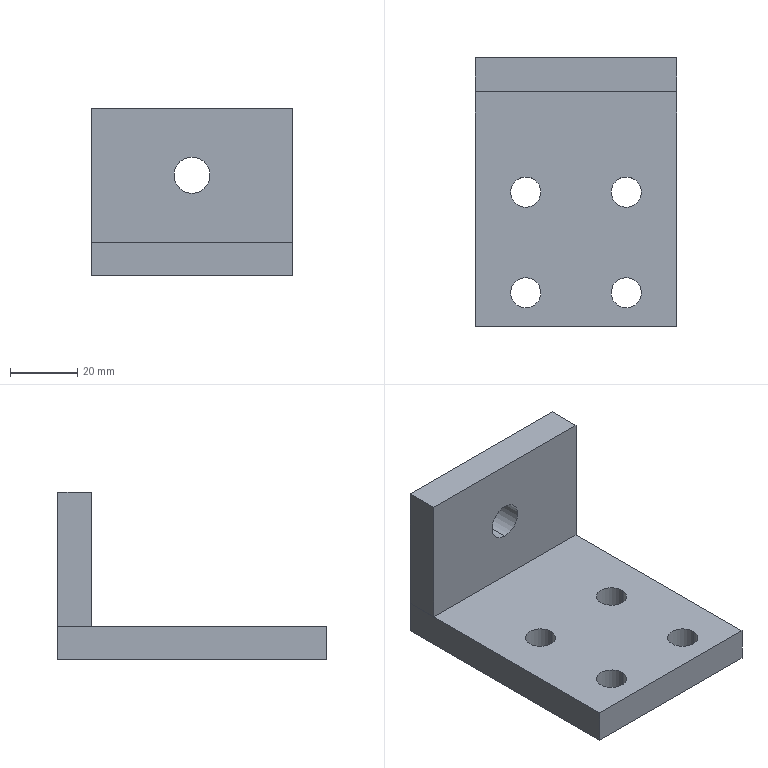Part | STEP file | 44-02-011 Press Platform Push Plate | 2 solids | 22 faces | box 60 x 80 x 50 mm | volume 68539 mm3 | plane 12 | cylinder 10 | commonest cylinder face diameters 9 x8 10.8 x2